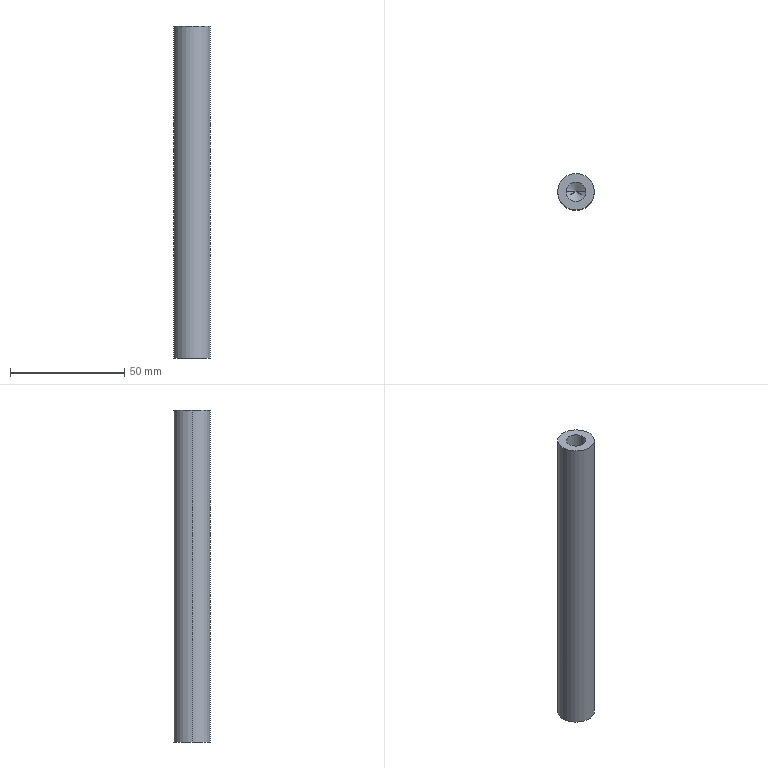Part | STEP file | B1-027 | 1 solid | 12 faces | box 16 x 16 x 145 mm | volume 27469 mm3 | cylinder 6 | cone 4 | plane 2 | commonest cylinder face diameters 8.5 x4 16 x2
STEP:
#1=CARTESIAN_POINT('',(0.,0.,0.));
#2=DIRECTION('',(0.,0.,1.));
#3=DIRECTION('',(1.,0.,0.));
#4=AXIS2_PLACEMENT_3D('',#1,#2,#3);
#5=CARTESIAN_POINT('',(4.25,0.,58.5));
#6=VERTEX_POINT('',#5);
#7=CARTESIAN_POINT('',(4.25,0.,72.5));
#8=VERTEX_POINT('',#7);
#9=CARTESIAN_POINT('',(4.25,0.,72.5));
#10=DIRECTION('',(0.,0.,1.));
#11=VECTOR('',#10,1.);
#12=LINE('',#9,#11);
#13=CARTESIAN_POINT('',(0.,0.,72.5));
#14=DIRECTION('',(0.,0.,1.));
#15=DIRECTION('',(1.,0.,0.));
#16=AXIS2_PLACEMENT_3D('',#13,#14,#15);
#17=CYLINDRICAL_SURFACE('',#16,4.25);
#18=CARTESIAN_POINT('',(6.283,0.));
#19=DIRECTION('',(0.,1.));
#20=VECTOR('',#19,1.);
#21=LINE('',#18,#20);
#22=(GEOMETRIC_REPRESENTATION_CONTEXT(2)PARAMETRIC_REPRESENTATION_CONTEXT()REPRESENTATION_CONTEXT('',''));
#23=DEFINITIONAL_REPRESENTATION('',(#21),#22);
#24=PCURVE('',#17,#23);
#25=CARTESIAN_POINT('',(0.,0.,72.5));
#26=DIRECTION('',(0.,0.,1.));
#27=DIRECTION('',(1.,0.,0.));
#28=AXIS2_PLACEMENT_3D('',#25,#26,#27);
#29=CYLINDRICAL_SURFACE('',#28,4.25);
#30=CARTESIAN_POINT('',(0.,0.));
#31=DIRECTION('',(0.,1.));
#32=VECTOR('',#31,1.);
#33=LINE('',#30,#32);
#34=(GEOMETRIC_REPRESENTATION_CONTEXT(2)PARAMETRIC_REPRESENTATION_CONTEXT()REPRESENTATION_CONTEXT('',''));
#35=DEFINITIONAL_REPRESENTATION('',(#33),#34);
#36=PCURVE('',#29,#35);
#37=SURFACE_CURVE('',#12,(#24,#36),.PCURVE_S1.);
#38=EDGE_CURVE('',#6,#8,#37,.T.);
#39=ORIENTED_EDGE('',*,*,#38,.T.);
#40=CARTESIAN_POINT('',(-4.25,0.,72.5));
#41=VERTEX_POINT('',#40);
#42=CARTESIAN_POINT('',(0.,0.,72.5));
#43=DIRECTION('',(0.,0.,1.));
#44=DIRECTION('',(1.,0.,0.));
#45=AXIS2_PLACEMENT_3D('',#42,#43,#44);
#46=CIRCLE('',#45,4.25);
#47=CARTESIAN_POINT('',(0.,0.));
#48=DIRECTION('',(1.,0.));
#49=VECTOR('',#48,1.);
#50=LINE('',#47,#49);
#51=(GEOMETRIC_REPRESENTATION_CONTEXT(2)PARAMETRIC_REPRESENTATION_CONTEXT()REPRESENTATION_CONTEXT('',''));
#52=DEFINITIONAL_REPRESENTATION('',(#50),#51);
#53=PCURVE('',#17,#52);
#54=CARTESIAN_POINT('',(0.,0.,72.5));
#55=DIRECTION('',(0.,0.,1.));
#56=DIRECTION('',(1.,0.,0.));
#57=AXIS2_PLACEMENT_3D('',#54,#55,#56);
#58=PLANE('',#57);
#59=CARTESIAN_POINT('',(0.,0.));
#60=DIRECTION('',(1.,0.));
#61=AXIS2_PLACEMENT_2D('',#59,#60);
#62=CIRCLE('',#61,4.25);
#63=(GEOMETRIC_REPRESENTATION_CONTEXT(2)PARAMETRIC_REPRESENTATION_CONTEXT()REPRESENTATION_CONTEXT('',''));
#64=DEFINITIONAL_REPRESENTATION('',(#62),#63);
#65=PCURVE('',#58,#64);
#66=SURFACE_CURVE('',#46,(#53,#65),.PCURVE_S1.);
#67=EDGE_CURVE('',#41,#8,#66,.T.);
#68=ORIENTED_EDGE('',*,*,#67,.F.);
#69=CARTESIAN_POINT('',(-4.25,0.,58.5));
#70=VERTEX_POINT('',#69);
#71=CARTESIAN_POINT('',(-4.25,0.,72.5));
#72=DIRECTION('',(0.,0.,1.));
#73=VECTOR('',#72,1.);
#74=LINE('',#71,#73);
#75=CARTESIAN_POINT('',(3.142,0.));
#76=DIRECTION('',(0.,1.));
#77=VECTOR('',#76,1.);
#78=LINE('',#75,#77);
#79=(GEOMETRIC_REPRESENTATION_CONTEXT(2)PARAMETRIC_REPRESENTATION_CONTEXT()REPRESENTATION_CONTEXT('',''));
#80=DEFINITIONAL_REPRESENTATION('',(#78),#79);
#81=PCURVE('',#17,#80);
#82=CARTESIAN_POINT('',(3.142,0.));
#83=DIRECTION('',(0.,1.));
#84=VECTOR('',#83,1.);
#85=LINE('',#82,#84);
#86=(GEOMETRIC_REPRESENTATION_CONTEXT(2)PARAMETRIC_REPRESENTATION_CONTEXT()REPRESENTATION_CONTEXT('',''));
#87=DEFINITIONAL_REPRESENTATION('',(#85),#86);
#88=PCURVE('',#29,#87);
#89=SURFACE_CURVE('',#74,(#81,#88),.PCURVE_S1.);
#90=EDGE_CURVE('',#70,#41,#89,.T.);
#91=ORIENTED_EDGE('',*,*,#90,.F.);
#92=CARTESIAN_POINT('',(0.,0.,58.5));
#93=DIRECTION('',(0.,0.,1.));
#94=DIRECTION('',(1.,0.,0.));
#95=AXIS2_PLACEMENT_3D('',#92,#93,#94);
#96=CIRCLE('',#95,4.25);
#97=CARTESIAN_POINT('',(0.,-14.));
#98=DIRECTION('',(1.,0.));
#99=VECTOR('',#98,1.);
#100=LINE('',#97,#99);
#101=(GEOMETRIC_REPRESENTATION_CONTEXT(2)PARAMETRIC_REPRESENTATION_CONTEXT()REPRESENTATION_CONTEXT('',''));
#102=DEFINITIONAL_REPRESENTATION('',(#100),#101);
#103=PCURVE('',#17,#102);
#104=CARTESIAN_POINT('',(0.,0.,58.5));
#105=DIRECTION('',(0.,0.,1.));
#106=DIRECTION('',(1.,0.,0.));
#107=AXIS2_PLACEMENT_3D('',#104,#105,#106);
#108=CONICAL_SURFACE('',#107,4.25,1.03);
#109=CARTESIAN_POINT('',(0.,0.));
#110=DIRECTION('',(1.,0.));
#111=VECTOR('',#110,1.);
#112=LINE('',#109,#111);
#113=(GEOMETRIC_REPRESENTATION_CONTEXT(2)PARAMETRIC_REPRESENTATION_CONTEXT()REPRESENTATION_CONTEXT('',''));
#114=DEFINITIONAL_REPRESENTATION('',(#112),#113);
#115=PCURVE('',#108,#114);
#116=SURFACE_CURVE('',#96,(#103,#115),.PCURVE_S1.);
#117=EDGE_CURVE('',#70,#6,#116,.T.);
#118=ORIENTED_EDGE('',*,*,#117,.T.);
#119=EDGE_LOOP('',(#39,#68,#91,#118));
#120=FACE_BOUND('',#119,.F.);
#121=ADVANCED_FACE('',(#120),#17,.F.);
#122=ORIENTED_EDGE('',*,*,#117,.F.);
#123=CARTESIAN_POINT('',(0.,0.,55.946));
#124=VERTEX_POINT('',#123);
#125=CARTESIAN_POINT('',(-4.25,0.,58.5));
#126=DIRECTION('',(-0.8572,0.,0.515));
#127=VECTOR('',#126,1.);
#128=LINE('',#125,#127);
#129=CARTESIAN_POINT('',(3.142,0.));
#130=DIRECTION('',(0.,1.));
#131=VECTOR('',#130,1.);
#132=LINE('',#129,#131);
#133=(GEOMETRIC_REPRESENTATION_CONTEXT(2)PARAMETRIC_REPRESENTATION_CONTEXT()REPRESENTATION_CONTEXT('',''));
#134=DEFINITIONAL_REPRESENTATION('',(#132),#133);
#135=PCURVE('',#108,#134);
#136=CARTESIAN_POINT('',(0.,0.,58.5));
#137=DIRECTION('',(0.,0.,1.));
#138=DIRECTION('',(1.,0.,0.));
#139=AXIS2_PLACEMENT_3D('',#136,#137,#138);
#140=CONICAL_SURFACE('',#139,4.25,1.03);
#141=CARTESIAN_POINT('',(3.142,0.));
#142=DIRECTION('',(0.,1.));
#143=VECTOR('',#142,1.);
#144=LINE('',#141,#143);
#145=(GEOMETRIC_REPRESENTATION_CONTEXT(2)PARAMETRIC_REPRESENTATION_CONTEXT()REPRESENTATION_CONTEXT('',''));
#146=DEFINITIONAL_REPRESENTATION('',(#144),#145);
#147=PCURVE('',#140,#146);
#148=SURFACE_CURVE('',#128,(#135,#147),.PCURVE_S1.);
#149=EDGE_CURVE('',#124,#70,#148,.T.);
#150=ORIENTED_EDGE('',*,*,#149,.F.);
#151=CARTESIAN_POINT('',(4.25,0.,58.5));
#152=DIRECTION('',(0.8572,0.,0.515));
#153=VECTOR('',#152,1.);
#154=LINE('',#151,#153);
#155=CARTESIAN_POINT('',(6.283,0.));
#156=DIRECTION('',(0.,1.));
#157=VECTOR('',#156,1.);
#158=LINE('',#155,#157);
#159=(GEOMETRIC_REPRESENTATION_CONTEXT(2)PARAMETRIC_REPRESENTATION_CONTEXT()REPRESENTATION_CONTEXT('',''));
#160=DEFINITIONAL_REPRESENTATION('',(#158),#159);
#161=PCURVE('',#108,#160);
#162=CARTESIAN_POINT('',(0.,0.));
#163=DIRECTION('',(0.,1.));
#164=VECTOR('',#163,1.);
#165=LINE('',#162,#164);
#166=(GEOMETRIC_REPRESENTATION_CONTEXT(2)PARAMETRIC_REPRESENTATION_CONTEXT()REPRESENTATION_CONTEXT('',''));
#167=DEFINITIONAL_REPRESENTATION('',(#165),#166);
#168=PCURVE('',#140,#167);
#169=SURFACE_CURVE('',#154,(#161,#168),.PCURVE_S1.);
#170=EDGE_CURVE('',#124,#6,#169,.T.);
#171=ORIENTED_EDGE('',*,*,#170,.T.);
#172=EDGE_LOOP('',(#122,#150,#171));
#173=FACE_BOUND('',#172,.F.);
#174=ADVANCED_FACE('',(#173),#108,.F.);
#175=CARTESIAN_POINT('',(-4.25,0.,-58.5));
#176=VERTEX_POINT('',#175);
#177=CARTESIAN_POINT('',(-4.25,0.,-72.5));
#178=VERTEX_POINT('',#177);
#179=CARTESIAN_POINT('',(-4.25,0.,-72.5));
#180=DIRECTION('',(0.,0.,-1.));
#181=VECTOR('',#180,1.);
#182=LINE('',#179,#181);
#183=CARTESIAN_POINT('',(0.,0.,-72.5));
#184=DIRECTION('',(0.,0.,-1.));
#185=DIRECTION('',(-1.,0.,0.));
#186=AXIS2_PLACEMENT_3D('',#183,#184,#185);
#187=CYLINDRICAL_SURFACE('',#186,4.25);
#188=CARTESIAN_POINT('',(6.283,0.));
#189=DIRECTION('',(0.,1.));
#190=VECTOR('',#189,1.);
#191=LINE('',#188,#190);
#192=(GEOMETRIC_REPRESENTATION_CONTEXT(2)PARAMETRIC_REPRESENTATION_CONTEXT()REPRESENTATION_CONTEXT('',''));
#193=DEFINITIONAL_REPRESENTATION('',(#191),#192);
#194=PCURVE('',#187,#193);
#195=CARTESIAN_POINT('',(0.,0.,-72.5));
#196=DIRECTION('',(0.,0.,-1.));
#197=DIRECTION('',(-1.,0.,0.));
#198=AXIS2_PLACEMENT_3D('',#195,#196,#197);
#199=CYLINDRICAL_SURFACE('',#198,4.25);
#200=CARTESIAN_POINT('',(0.,0.));
#201=DIRECTION('',(0.,1.));
#202=VECTOR('',#201,1.);
#203=LINE('',#200,#202);
#204=(GEOMETRIC_REPRESENTATION_CONTEXT(2)PARAMETRIC_REPRESENTATION_CONTEXT()REPRESENTATION_CONTEXT('',''));
#205=DEFINITIONAL_REPRESENTATION('',(#203),#204);
#206=PCURVE('',#199,#205);
#207=SURFACE_CURVE('',#182,(#194,#206),.PCURVE_S1.);
#208=EDGE_CURVE('',#176,#178,#207,.T.);
#209=ORIENTED_EDGE('',*,*,#208,.T.);
#210=CARTESIAN_POINT('',(4.25,0.,-72.5));
#211=VERTEX_POINT('',#210);
#212=CARTESIAN_POINT('',(0.,0.,-72.5));
#213=DIRECTION('',(0.,0.,-1.));
#214=DIRECTION('',(-1.,0.,0.));
#215=AXIS2_PLACEMENT_3D('',#212,#213,#214);
#216=CIRCLE('',#215,4.25);
#217=CARTESIAN_POINT('',(0.,0.));
#218=DIRECTION('',(1.,0.));
#219=VECTOR('',#218,1.);
#220=LINE('',#217,#219);
#221=(GEOMETRIC_REPRESENTATION_CONTEXT(2)PARAMETRIC_REPRESENTATION_CONTEXT()REPRESENTATION_CONTEXT('',''));
#222=DEFINITIONAL_REPRESENTATION('',(#220),#221);
#223=PCURVE('',#187,#222);
#224=CARTESIAN_POINT('',(0.,0.,-72.5));
#225=DIRECTION('',(0.,0.,1.));
#226=DIRECTION('',(1.,0.,0.));
#227=AXIS2_PLACEMENT_3D('',#224,#225,#226);
#228=PLANE('',#227);
#229=CARTESIAN_POINT('',(-4.25,0.));
#230=CARTESIAN_POINT('',(-4.25,7.361));
#231=CARTESIAN_POINT('',(2.125,3.681));
#232=CARTESIAN_POINT('',(8.5,0.));
#233=CARTESIAN_POINT('',(2.125,-3.681));
#234=CARTESIAN_POINT('',(-4.25,-7.361));
#235=CARTESIAN_POINT('',(-4.25,0.));
#236=(BOUNDED_CURVE()B_SPLINE_CURVE(2,(#229,#230,#231,#232,#233,#234,#235),.UNSPECIFIED.,.T.,.F.)B_SPLINE_CURVE_WITH_KNOTS((1,2,2,2,2,1),(-2.094,0.,2.094,4.189,6.283,8.378),.UNSPECIFIED.)CURVE()GEOMETRIC_REPRESENTATION_ITEM()RATIONAL_B_SPLINE_CURVE((1.,0.5,1.,0.5,1.,0.5,1.))REPRESENTATION_ITEM(''));
#237=(GEOMETRIC_REPRESENTATION_CONTEXT(2)PARAMETRIC_REPRESENTATION_CONTEXT()REPRESENTATION_CONTEXT('',''));
#238=DEFINITIONAL_REPRESENTATION('',(#236),#237);
#239=PCURVE('',#228,#238);
#240=SURFACE_CURVE('',#216,(#223,#239),.PCURVE_S1.);
#241=EDGE_CURVE('',#211,#178,#240,.T.);
#242=ORIENTED_EDGE('',*,*,#241,.F.);
#243=CARTESIAN_POINT('',(4.25,0.,-58.5));
#244=VERTEX_POINT('',#243);
#245=CARTESIAN_POINT('',(4.25,0.,-72.5));
#246=DIRECTION('',(0.,0.,-1.));
#247=VECTOR('',#246,1.);
#248=LINE('',#245,#247);
#249=CARTESIAN_POINT('',(3.142,0.));
#250=DIRECTION('',(0.,1.));
#251=VECTOR('',#250,1.);
#252=LINE('',#249,#251);
#253=(GEOMETRIC_REPRESENTATION_CONTEXT(2)PARAMETRIC_REPRESENTATION_CONTEXT()REPRESENTATION_CONTEXT('',''));
#254=DEFINITIONAL_REPRESENTATION('',(#252),#253);
#255=PCURVE('',#187,#254);
#256=CARTESIAN_POINT('',(3.142,0.));
#257=DIRECTION('',(0.,1.));
#258=VECTOR('',#257,1.);
#259=LINE('',#256,#258);
#260=(GEOMETRIC_REPRESENTATION_CONTEXT(2)PARAMETRIC_REPRESENTATION_CONTEXT()REPRESENTATION_CONTEXT('',''));
#261=DEFINITIONAL_REPRESENTATION('',(#259),#260);
#262=PCURVE('',#199,#261);
#263=SURFACE_CURVE('',#248,(#255,#262),.PCURVE_S1.);
#264=EDGE_CURVE('',#244,#211,#263,.T.);
#265=ORIENTED_EDGE('',*,*,#264,.F.);
#266=CARTESIAN_POINT('',(0.,0.,-58.5));
#267=DIRECTION('',(0.,0.,-1.));
#268=DIRECTION('',(-1.,0.,0.));
#269=AXIS2_PLACEMENT_3D('',#266,#267,#268);
#270=CIRCLE('',#269,4.25);
#271=CARTESIAN_POINT('',(0.,-14.));
#272=DIRECTION('',(1.,0.));
#273=VECTOR('',#272,1.);
#274=LINE('',#271,#273);
#275=(GEOMETRIC_REPRESENTATION_CONTEXT(2)PARAMETRIC_REPRESENTATION_CONTEXT()REPRESENTATION_CONTEXT('',''));
#276=DEFINITIONAL_REPRESENTATION('',(#274),#275);
#277=PCURVE('',#187,#276);
#278=CARTESIAN_POINT('',(0.,0.,-58.5));
#279=DIRECTION('',(0.,0.,-1.));
#280=DIRECTION('',(-1.,0.,0.));
#281=AXIS2_PLACEMENT_3D('',#278,#279,#280);
#282=CONICAL_SURFACE('',#281,4.25,1.03);
#283=CARTESIAN_POINT('',(0.,0.));
#284=DIRECTION('',(1.,0.));
#285=VECTOR('',#284,1.);
#286=LINE('',#283,#285);
#287=(GEOMETRIC_REPRESENTATION_CONTEXT(2)PARAMETRIC_REPRESENTATION_CONTEXT()REPRESENTATION_CONTEXT('',''));
#288=DEFINITIONAL_REPRESENTATION('',(#286),#287);
#289=PCURVE('',#282,#288);
#290=SURFACE_CURVE('',#270,(#277,#289),.PCURVE_S1.);
#291=EDGE_CURVE('',#244,#176,#290,.T.);
#292=ORIENTED_EDGE('',*,*,#291,.T.);
#293=EDGE_LOOP('',(#209,#242,#265,#292));
#294=FACE_BOUND('',#293,.F.);
#295=ADVANCED_FACE('',(#294),#187,.F.);
#296=ORIENTED_EDGE('',*,*,#291,.F.);
#297=CARTESIAN_POINT('',(0.,0.,-55.946));
#298=VERTEX_POINT('',#297);
#299=CARTESIAN_POINT('',(4.25,0.,-58.5));
#300=DIRECTION('',(0.8572,0.,-0.515));
#301=VECTOR('',#300,1.);
#302=LINE('',#299,#301);
#303=CARTESIAN_POINT('',(3.142,0.));
#304=DIRECTION('',(0.,1.));
#305=VECTOR('',#304,1.);
#306=LINE('',#303,#305);
#307=(GEOMETRIC_REPRESENTATION_CONTEXT(2)PARAMETRIC_REPRESENTATION_CONTEXT()REPRESENTATION_CONTEXT('',''));
#308=DEFINITIONAL_REPRESENTATION('',(#306),#307);
#309=PCURVE('',#282,#308);
#310=CARTESIAN_POINT('',(0.,0.,-58.5));
#311=DIRECTION('',(0.,0.,-1.));
#312=DIRECTION('',(-1.,0.,0.));
#313=AXIS2_PLACEMENT_3D('',#310,#311,#312);
#314=CONICAL_SURFACE('',#313,4.25,1.03);
#315=CARTESIAN_POINT('',(3.142,0.));
#316=DIRECTION('',(0.,1.));
#317=VECTOR('',#316,1.);
#318=LINE('',#315,#317);
#319=(GEOMETRIC_REPRESENTATION_CONTEXT(2)PARAMETRIC_REPRESENTATION_CONTEXT()REPRESENTATION_CONTEXT('',''));
#320=DEFINITIONAL_REPRESENTATION('',(#318),#319);
#321=PCURVE('',#314,#320);
#322=SURFACE_CURVE('',#302,(#309,#321),.PCURVE_S1.);
#323=EDGE_CURVE('',#298,#244,#322,.T.);
#324=ORIENTED_EDGE('',*,*,#323,.F.);
#325=CARTESIAN_POINT('',(-4.25,0.,-58.5));
#326=DIRECTION('',(-0.8572,0.,-0.515));
#327=VECTOR('',#326,1.);
#328=LINE('',#325,#327);
#329=CARTESIAN_POINT('',(6.283,0.));
#330=DIRECTION('',(0.,1.));
#331=VECTOR('',#330,1.);
#332=LINE('',#329,#331);
#333=(GEOMETRIC_REPRESENTATION_CONTEXT(2)PARAMETRIC_REPRESENTATION_CONTEXT()REPRESENTATION_CONTEXT('',''));
#334=DEFINITIONAL_REPRESENTATION('',(#332),#333);
#335=PCURVE('',#282,#334);
#336=CARTESIAN_POINT('',(0.,0.));
#337=DIRECTION('',(0.,1.));
#338=VECTOR('',#337,1.);
#339=LINE('',#336,#338);
#340=(GEOMETRIC_REPRESENTATION_CONTEXT(2)PARAMETRIC_REPRESENTATION_CONTEXT()REPRESENTATION_CONTEXT('',''));
#341=DEFINITIONAL_REPRESENTATION('',(#339),#340);
#342=PCURVE('',#314,#341);
#343=SURFACE_CURVE('',#328,(#335,#342),.PCURVE_S1.);
#344=EDGE_CURVE('',#298,#176,#343,.T.);
#345=ORIENTED_EDGE('',*,*,#344,.T.);
#346=EDGE_LOOP('',(#296,#324,#345));
#347=FACE_BOUND('',#346,.F.);
#348=ADVANCED_FACE('',(#347),#282,.F.);
#349=CARTESIAN_POINT('',(8.,0.,72.5));
#350=VERTEX_POINT('',#349);
#351=CARTESIAN_POINT('',(-8.,0.,72.5));
#352=VERTEX_POINT('',#351);
#353=CARTESIAN_POINT('',(0.,0.,72.5));
#354=DIRECTION('',(0.,0.,1.));
#355=DIRECTION('',(1.,0.,0.));
#356=AXIS2_PLACEMENT_3D('',#353,#354,#355);
#357=CIRCLE('',#356,8.);
#358=CARTESIAN_POINT('',(0.,0.,72.5));
#359=DIRECTION('',(0.,0.,-1.));
#360=DIRECTION('',(-1.,0.,0.));
#361=AXIS2_PLACEMENT_3D('',#358,#359,#360);
#362=CYLINDRICAL_SURFACE('',#361,8.);
#363=CARTESIAN_POINT('',(3.142,0.));
#364=DIRECTION('',(-1.,0.));
#365=VECTOR('',#364,1.);
#366=LINE('',#363,#365);
#367=(GEOMETRIC_REPRESENTATION_CONTEXT(2)PARAMETRIC_REPRESENTATION_CONTEXT()REPRESENTATION_CONTEXT('',''));
#368=DEFINITIONAL_REPRESENTATION('',(#366),#367);
#369=PCURVE('',#362,#368);
#370=CARTESIAN_POINT('',(0.,0.));
#371=DIRECTION('',(1.,0.));
#372=AXIS2_PLACEMENT_2D('',#370,#371);
#373=CIRCLE('',#372,8.);
#374=(GEOMETRIC_REPRESENTATION_CONTEXT(2)PARAMETRIC_REPRESENTATION_CONTEXT()REPRESENTATION_CONTEXT('',''));
#375=DEFINITIONAL_REPRESENTATION('',(#373),#374);
#376=PCURVE('',#58,#375);
#377=SURFACE_CURVE('',#357,(#369,#376),.PCURVE_S1.);
#378=EDGE_CURVE('',#350,#352,#377,.T.);
#379=ORIENTED_EDGE('',*,*,#378,.F.);
#380=CARTESIAN_POINT('',(8.,0.,-72.5));
#381=VERTEX_POINT('',#380);
#382=CARTESIAN_POINT('',(8.,0.,72.5));
#383=DIRECTION('',(0.,0.,-1.));
#384=VECTOR('',#383,1.);
#385=LINE('',#382,#384);
#386=CARTESIAN_POINT('',(3.142,0.));
#387=DIRECTION('',(0.,1.));
#388=VECTOR('',#387,1.);
#389=LINE('',#386,#388);
#390=(GEOMETRIC_REPRESENTATION_CONTEXT(2)PARAMETRIC_REPRESENTATION_CONTEXT()REPRESENTATION_CONTEXT('',''));
#391=DEFINITIONAL_REPRESENTATION('',(#389),#390);
#392=PCURVE('',#362,#391);
#393=CARTESIAN_POINT('',(0.,0.,72.5));
#394=DIRECTION('',(0.,0.,-1.));
#395=DIRECTION('',(-1.,0.,0.));
#396=AXIS2_PLACEMENT_3D('',#393,#394,#395);
#397=CYLINDRICAL_SURFACE('',#396,8.);
#398=CARTESIAN_POINT('',(3.142,0.));
#399=DIRECTION('',(0.,1.));
#400=VECTOR('',#399,1.);
#401=LINE('',#398,#400);
#402=(GEOMETRIC_REPRESENTATION_CONTEXT(2)PARAMETRIC_REPRESENTATION_CONTEXT()REPRESENTATION_CONTEXT('',''));
#403=DEFINITIONAL_REPRESENTATION('',(#401),#402);
#404=PCURVE('',#397,#403);
#405=SURFACE_CURVE('',#385,(#392,#404),.PCURVE_S1.);
#406=EDGE_CURVE('',#350,#381,#405,.T.);
#407=ORIENTED_EDGE('',*,*,#406,.T.);
#408=CARTESIAN_POINT('',(-8.,0.,-72.5));
#409=VERTEX_POINT('',#408);
#410=CARTESIAN_POINT('',(0.,0.,-72.5));
#411=DIRECTION('',(0.,0.,1.));
#412=DIRECTION('',(1.,0.,0.));
#413=AXIS2_PLACEMENT_3D('',#410,#411,#412);
#414=CIRCLE('',#413,8.);
#415=CARTESIAN_POINT('',(3.142,145.));
#416=DIRECTION('',(-1.,0.));
#417=VECTOR('',#416,1.);
#418=LINE('',#415,#417);
#419=(GEOMETRIC_REPRESENTATION_CONTEXT(2)PARAMETRIC_REPRESENTATION_CONTEXT()REPRESENTATION_CONTEXT('',''));
#420=DEFINITIONAL_REPRESENTATION('',(#418),#419);
#421=PCURVE('',#362,#420);
#422=CARTESIAN_POINT('',(0.,0.));
#423=DIRECTION('',(1.,0.));
#424=AXIS2_PLACEMENT_2D('',#422,#423);
#425=CIRCLE('',#424,8.);
#426=(GEOMETRIC_REPRESENTATION_CONTEXT(2)PARAMETRIC_REPRESENTATION_CONTEXT()REPRESENTATION_CONTEXT('',''));
#427=DEFINITIONAL_REPRESENTATION('',(#425),#426);
#428=PCURVE('',#228,#427);
#429=SURFACE_CURVE('',#414,(#421,#428),.PCURVE_S1.);
#430=EDGE_CURVE('',#381,#409,#429,.T.);
#431=ORIENTED_EDGE('',*,*,#430,.T.);
#432=CARTESIAN_POINT('',(-8.,0.,72.5));
#433=DIRECTION('',(0.,0.,-1.));
#434=VECTOR('',#433,1.);
#435=LINE('',#432,#434);
#436=CARTESIAN_POINT('',(0.,0.));
#437=DIRECTION('',(0.,1.));
#438=VECTOR('',#437,1.);
#439=LINE('',#436,#438);
#440=(GEOMETRIC_REPRESENTATION_CONTEXT(2)PARAMETRIC_REPRESENTATION_CONTEXT()REPRESENTATION_CONTEXT('',''));
#441=DEFINITIONAL_REPRESENTATION('',(#439),#440);
#442=PCURVE('',#362,#441);
#443=CARTESIAN_POINT('',(6.283,0.));
#444=DIRECTION('',(0.,1.));
#445=VECTOR('',#444,1.);
#446=LINE('',#443,#445);
#447=(GEOMETRIC_REPRESENTATION_CONTEXT(2)PARAMETRIC_REPRESENTATION_CONTEXT()REPRESENTATION_CONTEXT('',''));
#448=DEFINITIONAL_REPRESENTATION('',(#446),#447);
#449=PCURVE('',#397,#448);
#450=SURFACE_CURVE('',#435,(#442,#449),.PCURVE_S1.);
#451=EDGE_CURVE('',#352,#409,#450,.T.);
#452=ORIENTED_EDGE('',*,*,#451,.F.);
#453=EDGE_LOOP('',(#379,#407,#431,#452));
#454=FACE_BOUND('',#453,.T.);
#455=ADVANCED_FACE('',(#454),#362,.T.);
#456=ORIENTED_EDGE('',*,*,#406,.F.);
#457=CARTESIAN_POINT('',(0.,0.,72.5));
#458=DIRECTION('',(0.,0.,1.));
#459=DIRECTION('',(1.,0.,0.));
#460=AXIS2_PLACEMENT_3D('',#457,#458,#459);
#461=CIRCLE('',#460,8.);
#462=CARTESIAN_POINT('',(9.425,0.));
#463=DIRECTION('',(-1.,0.));
#464=VECTOR('',#463,1.);
#465=LINE('',#462,#464);
#466=(GEOMETRIC_REPRESENTATION_CONTEXT(2)PARAMETRIC_REPRESENTATION_CONTEXT()REPRESENTATION_CONTEXT('',''));
#467=DEFINITIONAL_REPRESENTATION('',(#465),#466);
#468=PCURVE('',#397,#467);
#469=CARTESIAN_POINT('',(0.,0.));
#470=DIRECTION('',(1.,0.));
#471=AXIS2_PLACEMENT_2D('',#469,#470);
#472=CIRCLE('',#471,8.);
#473=(GEOMETRIC_REPRESENTATION_CONTEXT(2)PARAMETRIC_REPRESENTATION_CONTEXT()REPRESENTATION_CONTEXT('',''));
#474=DEFINITIONAL_REPRESENTATION('',(#472),#473);
#475=PCURVE('',#58,#474);
#476=SURFACE_CURVE('',#461,(#468,#475),.PCURVE_S1.);
#477=EDGE_CURVE('',#352,#350,#476,.T.);
#478=ORIENTED_EDGE('',*,*,#477,.F.);
#479=ORIENTED_EDGE('',*,*,#451,.T.);
#480=CARTESIAN_POINT('',(0.,0.,-72.5));
#481=DIRECTION('',(0.,0.,1.));
#482=DIRECTION('',(1.,0.,0.));
#483=AXIS2_PLACEMENT_3D('',#480,#481,#482);
#484=CIRCLE('',#483,8.);
#485=CARTESIAN_POINT('',(9.425,145.));
#486=DIRECTION('',(-1.,0.));
#487=VECTOR('',#486,1.);
#488=LINE('',#485,#487);
#489=(GEOMETRIC_REPRESENTATION_CONTEXT(2)PARAMETRIC_REPRESENTATION_CONTEXT()REPRESENTATION_CONTEXT('',''));
#490=DEFINITIONAL_REPRESENTATION('',(#488),#489);
#491=PCURVE('',#397,#490);
#492=CARTESIAN_POINT('',(0.,0.));
#493=DIRECTION('',(1.,0.));
#494=AXIS2_PLACEMENT_2D('',#492,#493);
#495=CIRCLE('',#494,8.);
#496=(GEOMETRIC_REPRESENTATION_CONTEXT(2)PARAMETRIC_REPRESENTATION_CONTEXT()REPRESENTATION_CONTEXT('',''));
#497=DEFINITIONAL_REPRESENTATION('',(#495),#496);
#498=PCURVE('',#228,#497);
#499=SURFACE_CURVE('',#484,(#491,#498),.PCURVE_S1.);
#500=EDGE_CURVE('',#409,#381,#499,.T.);
#501=ORIENTED_EDGE('',*,*,#500,.T.);
#502=EDGE_LOOP('',(#456,#478,#479,#501));
#503=FACE_BOUND('',#502,.T.);
#504=ADVANCED_FACE('',(#503),#397,.T.);
#505=CARTESIAN_POINT('',(0.,0.,72.5));
#506=DIRECTION('',(0.,0.,1.));
#507=DIRECTION('',(1.,0.,0.));
#508=AXIS2_PLACEMENT_3D('',#505,#506,#507);
#509=CIRCLE('',#508,4.25);
#510=CARTESIAN_POINT('',(0.,0.));
#511=DIRECTION('',(1.,0.));
#512=AXIS2_PLACEMENT_2D('',#510,#511);
#513=CIRCLE('',#512,4.25);
#514=(GEOMETRIC_REPRESENTATION_CONTEXT(2)PARAMETRIC_REPRESENTATION_CONTEXT()REPRESENTATION_CONTEXT('',''));
#515=DEFINITIONAL_REPRESENTATION('',(#513),#514);
#516=PCURVE('',#58,#515);
#517=CARTESIAN_POINT('',(0.,0.));
#518=DIRECTION('',(1.,0.));
#519=VECTOR('',#518,1.);
#520=LINE('',#517,#519);
#521=(GEOMETRIC_REPRESENTATION_CONTEXT(2)PARAMETRIC_REPRESENTATION_CONTEXT()REPRESENTATION_CONTEXT('',''));
#522=DEFINITIONAL_REPRESENTATION('',(#520),#521);
#523=PCURVE('',#29,#522);
#524=SURFACE_CURVE('',#509,(#516,#523),.PCURVE_S1.);
#525=EDGE_CURVE('',#8,#41,#524,.T.);
#526=ORIENTED_EDGE('',*,*,#525,.F.);
#527=ORIENTED_EDGE('',*,*,#67,.F.);
#528=EDGE_LOOP('',(#526,#527));
#529=FACE_BOUND('',#528,.T.);
#530=ORIENTED_EDGE('',*,*,#477,.T.);
#531=ORIENTED_EDGE('',*,*,#378,.T.);
#532=EDGE_LOOP('',(#530,#531));
#533=FACE_BOUND('',#532,.T.);
#534=ADVANCED_FACE('',(#529,#533),#58,.T.);
#535=CARTESIAN_POINT('',(0.,0.,-72.5));
#536=DIRECTION('',(0.,0.,-1.));
#537=DIRECTION('',(-1.,0.,0.));
#538=AXIS2_PLACEMENT_3D('',#535,#536,#537);
#539=CIRCLE('',#538,4.25);
#540=CARTESIAN_POINT('',(-4.25,0.));
#541=CARTESIAN_POINT('',(-4.25,7.361));
#542=CARTESIAN_POINT('',(2.125,3.681));
#543=CARTESIAN_POINT('',(8.5,0.));
#544=CARTESIAN_POINT('',(2.125,-3.681));
#545=CARTESIAN_POINT('',(-4.25,-7.361));
#546=CARTESIAN_POINT('',(-4.25,0.));
#547=(BOUNDED_CURVE()B_SPLINE_CURVE(2,(#540,#541,#542,#543,#544,#545,#546),.UNSPECIFIED.,.T.,.F.)B_SPLINE_CURVE_WITH_KNOTS((1,2,2,2,2,1),(-2.094,0.,2.094,4.189,6.283,8.378),.UNSPECIFIED.)CURVE()GEOMETRIC_REPRESENTATION_ITEM()RATIONAL_B_SPLINE_CURVE((1.,0.5,1.,0.5,1.,0.5,1.))REPRESENTATION_ITEM(''));
#548=(GEOMETRIC_REPRESENTATION_CONTEXT(2)PARAMETRIC_REPRESENTATION_CONTEXT()REPRESENTATION_CONTEXT('',''));
#549=DEFINITIONAL_REPRESENTATION('',(#547),#548);
#550=PCURVE('',#228,#549);
#551=CARTESIAN_POINT('',(0.,0.));
#552=DIRECTION('',(1.,0.));
#553=VECTOR('',#552,1.);
#554=LINE('',#551,#553);
#555=(GEOMETRIC_REPRESENTATION_CONTEXT(2)PARAMETRIC_REPRESENTATION_CONTEXT()REPRESENTATION_CONTEXT('',''));
#556=DEFINITIONAL_REPRESENTATION('',(#554),#555);
#557=PCURVE('',#199,#556);
#558=SURFACE_CURVE('',#539,(#550,#557),.PCURVE_S1.);
#559=EDGE_CURVE('',#178,#211,#558,.T.);
#560=ORIENTED_EDGE('',*,*,#559,.F.);
#561=ORIENTED_EDGE('',*,*,#241,.F.);
#562=EDGE_LOOP('',(#560,#561));
#563=FACE_BOUND('',#562,.T.);
#564=ORIENTED_EDGE('',*,*,#500,.F.);
#565=ORIENTED_EDGE('',*,*,#430,.F.);
#566=EDGE_LOOP('',(#564,#565));
#567=FACE_BOUND('',#566,.T.);
#568=ADVANCED_FACE('',(#563,#567),#228,.F.);
#569=CARTESIAN_POINT('',(0.,0.,-58.5));
#570=DIRECTION('',(0.,0.,-1.));
#571=DIRECTION('',(-1.,0.,0.));
#572=AXIS2_PLACEMENT_3D('',#569,#570,#571);
#573=CIRCLE('',#572,4.25);
#574=CARTESIAN_POINT('',(0.,0.));
#575=DIRECTION('',(1.,0.));
#576=VECTOR('',#575,1.);
#577=LINE('',#574,#576);
#578=(GEOMETRIC_REPRESENTATION_CONTEXT(2)PARAMETRIC_REPRESENTATION_CONTEXT()REPRESENTATION_CONTEXT('',''));
#579=DEFINITIONAL_REPRESENTATION('',(#577),#578);
#580=PCURVE('',#314,#579);
#581=CARTESIAN_POINT('',(0.,-14.));
#582=DIRECTION('',(1.,0.));
#583=VECTOR('',#582,1.);
#584=LINE('',#581,#583);
#585=(GEOMETRIC_REPRESENTATION_CONTEXT(2)PARAMETRIC_REPRESENTATION_CONTEXT()REPRESENTATION_CONTEXT('',''));
#586=DEFINITIONAL_REPRESENTATION('',(#584),#585);
#587=PCURVE('',#199,#586);
#588=SURFACE_CURVE('',#573,(#580,#587),.PCURVE_S1.);
#589=EDGE_CURVE('',#176,#244,#588,.T.);
#590=ORIENTED_EDGE('',*,*,#589,.F.);
#591=ORIENTED_EDGE('',*,*,#344,.F.);
#592=ORIENTED_EDGE('',*,*,#323,.T.);
#593=EDGE_LOOP('',(#590,#591,#592));
#594=FACE_BOUND('',#593,.F.);
#595=ADVANCED_FACE('',(#594),#314,.F.);
#596=ORIENTED_EDGE('',*,*,#559,.F.);
#597=ORIENTED_EDGE('',*,*,#208,.F.);
#598=ORIENTED_EDGE('',*,*,#589,.T.);
#599=ORIENTED_EDGE('',*,*,#264,.T.);
#600=EDGE_LOOP('',(#596,#597,#598,#599));
#601=FACE_BOUND('',#600,.F.);
#602=ADVANCED_FACE('',(#601),#199,.F.);
#603=CARTESIAN_POINT('',(0.,0.,58.5));
#604=DIRECTION('',(0.,0.,1.));
#605=DIRECTION('',(1.,0.,0.));
#606=AXIS2_PLACEMENT_3D('',#603,#604,#605);
#607=CIRCLE('',#606,4.25);
#608=CARTESIAN_POINT('',(0.,0.));
#609=DIRECTION('',(1.,0.));
#610=VECTOR('',#609,1.);
#611=LINE('',#608,#610);
#612=(GEOMETRIC_REPRESENTATION_CONTEXT(2)PARAMETRIC_REPRESENTATION_CONTEXT()REPRESENTATION_CONTEXT('',''));
#613=DEFINITIONAL_REPRESENTATION('',(#611),#612);
#614=PCURVE('',#140,#613);
#615=CARTESIAN_POINT('',(0.,-14.));
#616=DIRECTION('',(1.,0.));
#617=VECTOR('',#616,1.);
#618=LINE('',#615,#617);
#619=(GEOMETRIC_REPRESENTATION_CONTEXT(2)PARAMETRIC_REPRESENTATION_CONTEXT()REPRESENTATION_CONTEXT('',''));
#620=DEFINITIONAL_REPRESENTATION('',(#618),#619);
#621=PCURVE('',#29,#620);
#622=SURFACE_CURVE('',#607,(#614,#621),.PCURVE_S1.);
#623=EDGE_CURVE('',#6,#70,#622,.T.);
#624=ORIENTED_EDGE('',*,*,#623,.F.);
#625=ORIENTED_EDGE('',*,*,#170,.F.);
#626=ORIENTED_EDGE('',*,*,#149,.T.);
#627=EDGE_LOOP('',(#624,#625,#626));
#628=FACE_BOUND('',#627,.F.);
#629=ADVANCED_FACE('',(#628),#140,.F.);
#630=ORIENTED_EDGE('',*,*,#525,.F.);
#631=ORIENTED_EDGE('',*,*,#38,.F.);
#632=ORIENTED_EDGE('',*,*,#623,.T.);
#633=ORIENTED_EDGE('',*,*,#90,.T.);
#634=EDGE_LOOP('',(#630,#631,#632,#633));
#635=FACE_BOUND('',#634,.F.);
#636=ADVANCED_FACE('',(#635),#29,.F.);
#637=CLOSED_SHELL('',(#121,#174,#295,#348,#455,#504,#534,#568,#595,#602,#629,#636));
#638=MANIFOLD_SOLID_BREP('',#637);
#639=(LENGTH_UNIT()NAMED_UNIT(*)SI_UNIT(.MILLI.,.METRE.));
#640=UNCERTAINTY_MEASURE_WITH_UNIT(LENGTH_MEASURE(0.0000001),#639,'','');
#641=(NAMED_UNIT(*)PLANE_ANGLE_UNIT()SI_UNIT($,.RADIAN.));
#642=(NAMED_UNIT(*)SI_UNIT($,.STERADIAN.)SOLID_ANGLE_UNIT());
#643=(GEOMETRIC_REPRESENTATION_CONTEXT(3)GLOBAL_UNCERTAINTY_ASSIGNED_CONTEXT((#640))GLOBAL_UNIT_ASSIGNED_CONTEXT((#639,#641,#642))REPRESENTATION_CONTEXT('',''));
#644=ADVANCED_BREP_SHAPE_REPRESENTATION('',(#4,#638),#643);